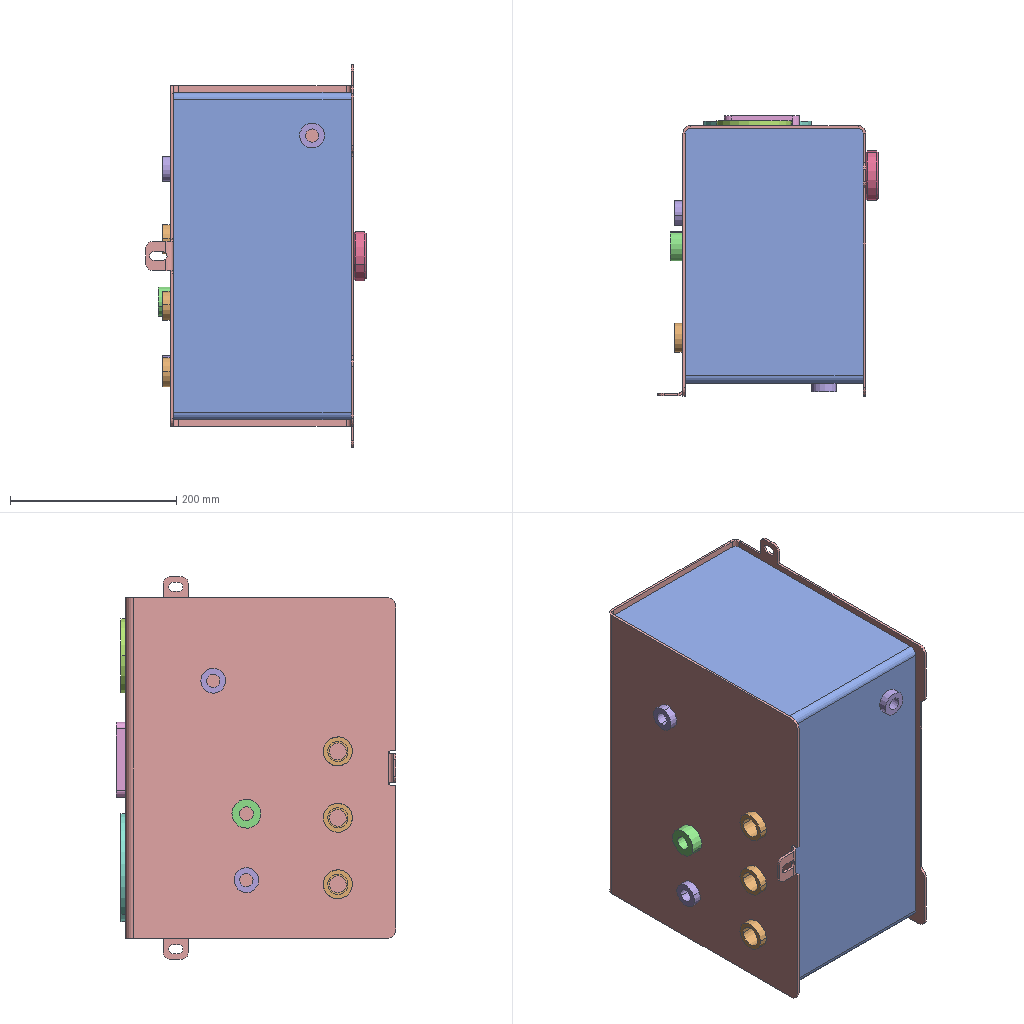Assembly | SolidWorks | 9 different items | 13 placed | box 265 x 337 x 460 mm
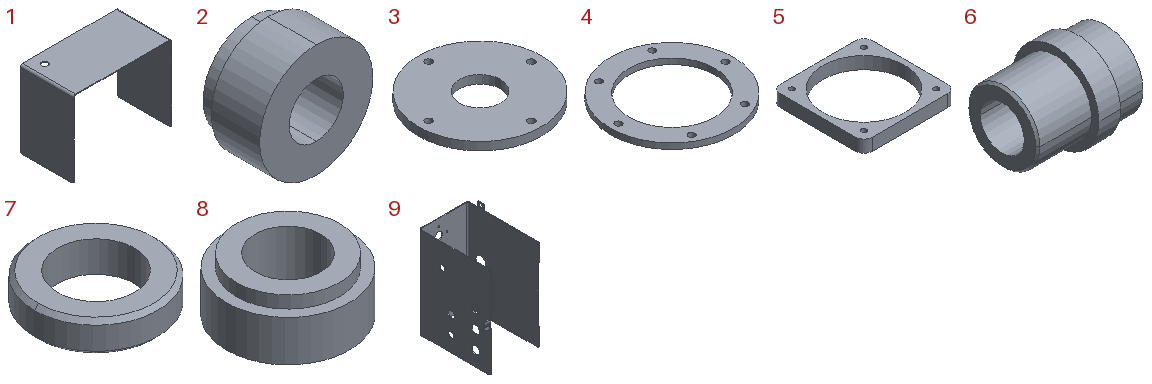Parts list (item | quantity | size | volume | features):
1 | x1 | 394 x 214 x 307 mm | 637569 mm3 | features Fillet 1, FlatPattern 1, ICE 1, SMBaseFlange 1, SheetMetal 1
2 | x1 | 35 x 20 x 35 mm | 13533 mm3 | features ICE 2, Extrusion 1
3 | x1 | 90 x 90 x 6 mm | 33458 mm3 | features FlatPattern 1, HoleWzd 1, SMBaseFlange 1, SheetMetal 1
4 | x1 | 130 x 130 x 6 mm | 40162 mm3 | features FlatPattern 1, HoleWzd 1, SMBaseFlange 1, SheetMetal 1
5 | x1 | 90 x 90 x 12 mm | 35280 mm3 | features FlatPattern 1, HoleWzd 1, SMBaseFlange 1, SheetMetal 1
6 | x3 | 48 x 40 x 40 mm | 27829 mm3 | features ICE 2, Revolution 1
7 | x1 | 60 x 60 x 15 mm | 25107 mm3 | features Chamfer 1, Extrusion 1, HoleWzd 1, ICE 1
8 | x3 | 30 x 30 x 13 mm | 5927 mm3 | features ICE 2, Extrusion 1
9 | x1 | 250 x 325 x 460 mm | 996726 mm3 | features ICE 8, Fillet 5, EdgeFlange 1, FlatPattern 1, SMBaseFlange 1, SheetMetal 1
Mates (type | each side: item.copy, entity, surface, feature):
Coincident | 9.1 face plane Base-Flange1 | 1.1 face plane Base-Flange1 | 2 times
DistanceDim | 1.1 face plane Base-Flange1 | 9.1 face plane Cut-Extrude2
Coincident | 9.1 face plane Base-Flange1 | 3.1 face plane Base-Flange1
Concentric | 9.1 edge | 3.1 edge | 2 times
Coincident | 9.1 face plane Base-Flange1 | 5.1 face plane Base-Flange1
Concentric | 9.1 edge | 5.1 edge
Parallel | 9.1 face plane Base-Flange1 | 5.1 face plane Base-Flange1
Coincident | 9.1 face plane Base-Flange1 | 4.1 face plane Base-Flange1
Concentric | 9.1 edge | 4.1 edge | 2 times
Coincident | 6.1 face plane Revolve1 | 6.2 face plane Revolve1
Concentric | 9.1 edge | 6.1 edge
Concentric | 9.1 edge | 6.2 edge
Concentric | 9.1 edge | 6.3 edge
Coincident | 9.1 face plane Base-Flange1 | 6.3 face plane Revolve1
Coincident | 6.3 face plane Revolve1 | 6.2 face plane Revolve1
Coincident | assembly face | assembly face
Coincident | 9.1 face plane Base-Flange1 | assembly face
Coincident | 8.1 face plane Boss-Extrude1 | 8.2 face plane Boss-Extrude1
Concentric | 9.1 edge | 8.1 edge
Coincident | 9.1 face plane Base-Flange1 | 8.1 face plane Boss-Extrude1
Concentric | 9.1 edge | 8.2 edge
Coincident | 9.1 face plane Base-Flange1 | 2.1 face plane Boss-Extrude1
Concentric | 9.1 edge | 2.1 edge
Coincident | 9.1 face plane Base-Flange1 | 7.1 face plane Boss-Extrude1
Coincident | 1.1 face plane Base-Flange1 | 8.3 face plane Boss-Extrude1
Concentric | 1.1 edge | 8.3 edge